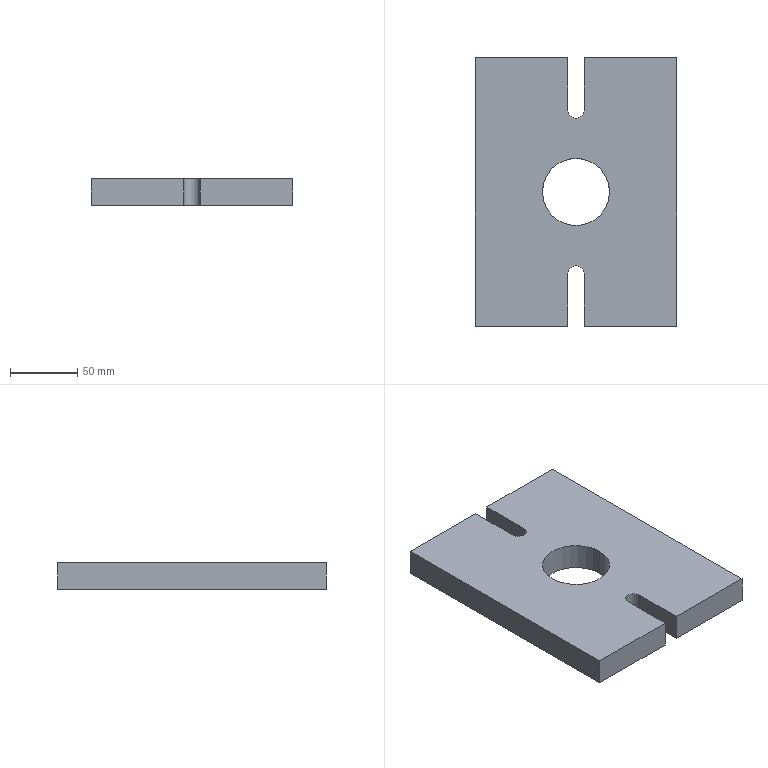Part | SolidWorks | features Extrusion 1 | 1 solid | 16 faces | box 150 x 200 x 20 mm | volume 539748 mm3 | plane 12 | cylinder 4 | commonest cylinder face diameters 12 x2 50 x2
STEP:
#1=CARTESIAN_POINT('',(50.,100.,20.));
#2=VERTEX_POINT('',#1);
#3=CARTESIAN_POINT('',(100.,100.,20.));
#4=VERTEX_POINT('',#3);
#5=CARTESIAN_POINT('',(75.,100.,20.));
#6=DIRECTION('',(0.,0.,1.));
#7=DIRECTION('',(1.,0.,0.));
#8=AXIS2_PLACEMENT_3D('',#5,#6,#7);
#9=CIRCLE('',#8,25.);
#10=EDGE_CURVE('',#2,#4,#9,.T.);
#11=ORIENTED_EDGE('',*,*,#10,.T.);
#12=CARTESIAN_POINT('',(100.,100.,0.));
#13=VERTEX_POINT('',#12);
#14=CARTESIAN_POINT('',(100.,100.,20.));
#15=DIRECTION('',(0.,0.,-1.));
#16=VECTOR('',#15,1000.);
#17=LINE('',#14,#16);
#18=EDGE_CURVE('',#4,#13,#17,.T.);
#19=ORIENTED_EDGE('',*,*,#18,.T.);
#20=CARTESIAN_POINT('',(50.,100.,0.));
#21=VERTEX_POINT('',#20);
#22=CARTESIAN_POINT('',(75.,100.,0.));
#23=DIRECTION('',(0.,0.,1.));
#24=DIRECTION('',(1.,0.,0.));
#25=AXIS2_PLACEMENT_3D('',#22,#23,#24);
#26=CIRCLE('',#25,25.);
#27=EDGE_CURVE('',#21,#13,#26,.T.);
#28=ORIENTED_EDGE('',*,*,#27,.F.);
#29=CARTESIAN_POINT('',(50.,100.,20.));
#30=DIRECTION('',(0.,0.,-1.));
#31=VECTOR('',#30,1000.);
#32=LINE('',#29,#31);
#33=EDGE_CURVE('',#2,#21,#32,.T.);
#34=ORIENTED_EDGE('',*,*,#33,.F.);
#35=EDGE_LOOP('',(#11,#19,#28,#34));
#36=FACE_OUTER_BOUND('',#35,.T.);
#37=CARTESIAN_POINT('',(75.,100.,20.));
#38=DIRECTION('',(0.,0.,-1.));
#39=DIRECTION('',(-1.,0.,0.));
#40=AXIS2_PLACEMENT_3D('',#37,#38,#39);
#41=CYLINDRICAL_SURFACE('',#40,25.);
#42=ADVANCED_FACE('',(#36),#41,.F.);
#43=CARTESIAN_POINT('',(0.,200.,20.));
#44=VERTEX_POINT('',#43);
#45=CARTESIAN_POINT('',(0.,0.,20.));
#46=VERTEX_POINT('',#45);
#47=CARTESIAN_POINT('',(0.,0.,20.));
#48=DIRECTION('',(0.,-1.,0.));
#49=VECTOR('',#48,1000.);
#50=LINE('',#47,#49);
#51=EDGE_CURVE('',#44,#46,#50,.T.);
#52=ORIENTED_EDGE('',*,*,#51,.T.);
#53=CARTESIAN_POINT('',(69.,0.,20.));
#54=VERTEX_POINT('',#53);
#55=CARTESIAN_POINT('',(0.,0.,20.));
#56=DIRECTION('',(1.,0.,0.));
#57=VECTOR('',#56,1000.);
#58=LINE('',#55,#57);
#59=EDGE_CURVE('',#46,#54,#58,.T.);
#60=ORIENTED_EDGE('',*,*,#59,.T.);
#61=CARTESIAN_POINT('',(69.,39.,20.));
#62=VERTEX_POINT('',#61);
#63=CARTESIAN_POINT('',(69.,0.,20.));
#64=DIRECTION('',(0.,1.,0.));
#65=VECTOR('',#64,1000.);
#66=LINE('',#63,#65);
#67=EDGE_CURVE('',#54,#62,#66,.T.);
#68=ORIENTED_EDGE('',*,*,#67,.T.);
#69=CARTESIAN_POINT('',(81.,39.,20.));
#70=VERTEX_POINT('',#69);
#71=CARTESIAN_POINT('',(75.,39.,20.));
#72=DIRECTION('',(0.,0.,-1.));
#73=DIRECTION('',(-1.,0.,0.));
#74=AXIS2_PLACEMENT_3D('',#71,#72,#73);
#75=CIRCLE('',#74,6.);
#76=EDGE_CURVE('',#62,#70,#75,.T.);
#77=ORIENTED_EDGE('',*,*,#76,.T.);
#78=CARTESIAN_POINT('',(81.,0.,20.));
#79=VERTEX_POINT('',#78);
#80=CARTESIAN_POINT('',(81.,39.,20.));
#81=DIRECTION('',(0.,-1.,0.));
#82=VECTOR('',#81,1000.);
#83=LINE('',#80,#82);
#84=EDGE_CURVE('',#70,#79,#83,.T.);
#85=ORIENTED_EDGE('',*,*,#84,.T.);
#86=CARTESIAN_POINT('',(150.,0.,20.));
#87=VERTEX_POINT('',#86);
#88=CARTESIAN_POINT('',(81.,0.,20.));
#89=DIRECTION('',(1.,0.,0.));
#90=VECTOR('',#89,1000.);
#91=LINE('',#88,#90);
#92=EDGE_CURVE('',#79,#87,#91,.T.);
#93=ORIENTED_EDGE('',*,*,#92,.T.);
#94=CARTESIAN_POINT('',(150.,200.,20.));
#95=VERTEX_POINT('',#94);
#96=CARTESIAN_POINT('',(150.,0.,20.));
#97=DIRECTION('',(0.,1.,0.));
#98=VECTOR('',#97,1000.);
#99=LINE('',#96,#98);
#100=EDGE_CURVE('',#87,#95,#99,.T.);
#101=ORIENTED_EDGE('',*,*,#100,.T.);
#102=CARTESIAN_POINT('',(81.,200.,20.));
#103=VERTEX_POINT('',#102);
#104=CARTESIAN_POINT('',(81.,200.,20.));
#105=DIRECTION('',(-1.,0.,0.));
#106=VECTOR('',#105,1000.);
#107=LINE('',#104,#106);
#108=EDGE_CURVE('',#95,#103,#107,.T.);
#109=ORIENTED_EDGE('',*,*,#108,.T.);
#110=CARTESIAN_POINT('',(81.,161.,20.));
#111=VERTEX_POINT('',#110);
#112=CARTESIAN_POINT('',(81.,161.,20.));
#113=DIRECTION('',(0.,-1.,0.));
#114=VECTOR('',#113,1000.);
#115=LINE('',#112,#114);
#116=EDGE_CURVE('',#103,#111,#115,.T.);
#117=ORIENTED_EDGE('',*,*,#116,.T.);
#118=CARTESIAN_POINT('',(69.,161.,20.));
#119=VERTEX_POINT('',#118);
#120=CARTESIAN_POINT('',(75.,161.,20.));
#121=DIRECTION('',(0.,0.,-1.));
#122=DIRECTION('',(1.,0.,0.));
#123=AXIS2_PLACEMENT_3D('',#120,#121,#122);
#124=CIRCLE('',#123,6.);
#125=EDGE_CURVE('',#111,#119,#124,.T.);
#126=ORIENTED_EDGE('',*,*,#125,.T.);
#127=CARTESIAN_POINT('',(69.,200.,20.));
#128=VERTEX_POINT('',#127);
#129=CARTESIAN_POINT('',(69.,200.,20.));
#130=DIRECTION('',(0.,1.,0.));
#131=VECTOR('',#130,1000.);
#132=LINE('',#129,#131);
#133=EDGE_CURVE('',#119,#128,#132,.T.);
#134=ORIENTED_EDGE('',*,*,#133,.T.);
#135=CARTESIAN_POINT('',(0.,200.,20.));
#136=DIRECTION('',(-1.,0.,0.));
#137=VECTOR('',#136,1000.);
#138=LINE('',#135,#137);
#139=EDGE_CURVE('',#128,#44,#138,.T.);
#140=ORIENTED_EDGE('',*,*,#139,.T.);
#141=EDGE_LOOP('',(#52,#60,#68,#77,#85,#93,#101,#109,#117,#126,#134,#140));
#142=FACE_OUTER_BOUND('',#141,.T.);
#143=ORIENTED_EDGE('',*,*,#10,.F.);
#144=CARTESIAN_POINT('',(75.,100.,20.));
#145=DIRECTION('',(0.,0.,1.));
#146=DIRECTION('',(1.,0.,0.));
#147=AXIS2_PLACEMENT_3D('',#144,#145,#146);
#148=CIRCLE('',#147,25.);
#149=EDGE_CURVE('',#4,#2,#148,.T.);
#150=ORIENTED_EDGE('',*,*,#149,.F.);
#151=EDGE_LOOP('',(#143,#150));
#152=FACE_BOUND('',#151,.T.);
#153=CARTESIAN_POINT('',(75.,161.,20.));
#154=DIRECTION('',(0.,0.,1.));
#155=DIRECTION('',(1.,0.,0.));
#156=AXIS2_PLACEMENT_3D('',#153,#154,#155);
#157=PLANE('',#156);
#158=ADVANCED_FACE('',(#142,#152),#157,.T.);
#159=CARTESIAN_POINT('',(0.,200.,0.));
#160=VERTEX_POINT('',#159);
#161=CARTESIAN_POINT('',(0.,0.,0.));
#162=VERTEX_POINT('',#161);
#163=CARTESIAN_POINT('',(0.,0.,0.));
#164=DIRECTION('',(0.,-1.,0.));
#165=VECTOR('',#164,1000.);
#166=LINE('',#163,#165);
#167=EDGE_CURVE('',#160,#162,#166,.T.);
#168=ORIENTED_EDGE('',*,*,#167,.F.);
#169=CARTESIAN_POINT('',(69.,200.,0.));
#170=VERTEX_POINT('',#169);
#171=CARTESIAN_POINT('',(0.,200.,0.));
#172=DIRECTION('',(-1.,0.,0.));
#173=VECTOR('',#172,1000.);
#174=LINE('',#171,#173);
#175=EDGE_CURVE('',#170,#160,#174,.T.);
#176=ORIENTED_EDGE('',*,*,#175,.F.);
#177=CARTESIAN_POINT('',(69.,161.,0.));
#178=VERTEX_POINT('',#177);
#179=CARTESIAN_POINT('',(69.,200.,0.));
#180=DIRECTION('',(0.,1.,0.));
#181=VECTOR('',#180,1000.);
#182=LINE('',#179,#181);
#183=EDGE_CURVE('',#178,#170,#182,.T.);
#184=ORIENTED_EDGE('',*,*,#183,.F.);
#185=CARTESIAN_POINT('',(81.,161.,0.));
#186=VERTEX_POINT('',#185);
#187=CARTESIAN_POINT('',(75.,161.,0.));
#188=DIRECTION('',(0.,0.,-1.));
#189=DIRECTION('',(1.,0.,0.));
#190=AXIS2_PLACEMENT_3D('',#187,#188,#189);
#191=CIRCLE('',#190,6.);
#192=EDGE_CURVE('',#186,#178,#191,.T.);
#193=ORIENTED_EDGE('',*,*,#192,.F.);
#194=CARTESIAN_POINT('',(81.,200.,0.));
#195=VERTEX_POINT('',#194);
#196=CARTESIAN_POINT('',(81.,161.,0.));
#197=DIRECTION('',(0.,-1.,0.));
#198=VECTOR('',#197,1000.);
#199=LINE('',#196,#198);
#200=EDGE_CURVE('',#195,#186,#199,.T.);
#201=ORIENTED_EDGE('',*,*,#200,.F.);
#202=CARTESIAN_POINT('',(150.,200.,0.));
#203=VERTEX_POINT('',#202);
#204=CARTESIAN_POINT('',(81.,200.,0.));
#205=DIRECTION('',(-1.,0.,0.));
#206=VECTOR('',#205,1000.);
#207=LINE('',#204,#206);
#208=EDGE_CURVE('',#203,#195,#207,.T.);
#209=ORIENTED_EDGE('',*,*,#208,.F.);
#210=CARTESIAN_POINT('',(150.,0.,0.));
#211=VERTEX_POINT('',#210);
#212=CARTESIAN_POINT('',(150.,0.,0.));
#213=DIRECTION('',(0.,1.,0.));
#214=VECTOR('',#213,1000.);
#215=LINE('',#212,#214);
#216=EDGE_CURVE('',#211,#203,#215,.T.);
#217=ORIENTED_EDGE('',*,*,#216,.F.);
#218=CARTESIAN_POINT('',(81.,0.,0.));
#219=VERTEX_POINT('',#218);
#220=CARTESIAN_POINT('',(81.,0.,0.));
#221=DIRECTION('',(1.,0.,0.));
#222=VECTOR('',#221,1000.);
#223=LINE('',#220,#222);
#224=EDGE_CURVE('',#219,#211,#223,.T.);
#225=ORIENTED_EDGE('',*,*,#224,.F.);
#226=CARTESIAN_POINT('',(81.,39.,0.));
#227=VERTEX_POINT('',#226);
#228=CARTESIAN_POINT('',(81.,39.,0.));
#229=DIRECTION('',(0.,-1.,0.));
#230=VECTOR('',#229,1000.);
#231=LINE('',#228,#230);
#232=EDGE_CURVE('',#227,#219,#231,.T.);
#233=ORIENTED_EDGE('',*,*,#232,.F.);
#234=CARTESIAN_POINT('',(69.,39.,0.));
#235=VERTEX_POINT('',#234);
#236=CARTESIAN_POINT('',(75.,39.,0.));
#237=DIRECTION('',(0.,0.,-1.));
#238=DIRECTION('',(-1.,0.,0.));
#239=AXIS2_PLACEMENT_3D('',#236,#237,#238);
#240=CIRCLE('',#239,6.);
#241=EDGE_CURVE('',#235,#227,#240,.T.);
#242=ORIENTED_EDGE('',*,*,#241,.F.);
#243=CARTESIAN_POINT('',(69.,0.,0.));
#244=VERTEX_POINT('',#243);
#245=CARTESIAN_POINT('',(69.,0.,0.));
#246=DIRECTION('',(0.,1.,0.));
#247=VECTOR('',#246,1000.);
#248=LINE('',#245,#247);
#249=EDGE_CURVE('',#244,#235,#248,.T.);
#250=ORIENTED_EDGE('',*,*,#249,.F.);
#251=CARTESIAN_POINT('',(0.,0.,0.));
#252=DIRECTION('',(1.,0.,0.));
#253=VECTOR('',#252,1000.);
#254=LINE('',#251,#253);
#255=EDGE_CURVE('',#162,#244,#254,.T.);
#256=ORIENTED_EDGE('',*,*,#255,.F.);
#257=EDGE_LOOP('',(#168,#176,#184,#193,#201,#209,#217,#225,#233,#242,#250,#256));
#258=FACE_OUTER_BOUND('',#257,.T.);
#259=ORIENTED_EDGE('',*,*,#27,.T.);
#260=CARTESIAN_POINT('',(75.,100.,0.));
#261=DIRECTION('',(0.,0.,1.));
#262=DIRECTION('',(1.,0.,0.));
#263=AXIS2_PLACEMENT_3D('',#260,#261,#262);
#264=CIRCLE('',#263,25.);
#265=EDGE_CURVE('',#13,#21,#264,.T.);
#266=ORIENTED_EDGE('',*,*,#265,.T.);
#267=EDGE_LOOP('',(#259,#266));
#268=FACE_BOUND('',#267,.T.);
#269=CARTESIAN_POINT('',(75.,161.,0.));
#270=DIRECTION('',(0.,0.,1.));
#271=DIRECTION('',(1.,0.,0.));
#272=AXIS2_PLACEMENT_3D('',#269,#270,#271);
#273=PLANE('',#272);
#274=ADVANCED_FACE('',(#258,#268),#273,.F.);
#275=ORIENTED_EDGE('',*,*,#167,.T.);
#276=CARTESIAN_POINT('',(0.,0.,20.));
#277=DIRECTION('',(0.,0.,-1.));
#278=VECTOR('',#277,1000.);
#279=LINE('',#276,#278);
#280=EDGE_CURVE('',#46,#162,#279,.T.);
#281=ORIENTED_EDGE('',*,*,#280,.F.);
#282=ORIENTED_EDGE('',*,*,#51,.F.);
#283=CARTESIAN_POINT('',(0.,200.,20.));
#284=DIRECTION('',(0.,0.,-1.));
#285=VECTOR('',#284,1000.);
#286=LINE('',#283,#285);
#287=EDGE_CURVE('',#44,#160,#286,.T.);
#288=ORIENTED_EDGE('',*,*,#287,.T.);
#289=EDGE_LOOP('',(#275,#281,#282,#288));
#290=FACE_OUTER_BOUND('',#289,.T.);
#291=CARTESIAN_POINT('',(0.,0.,20.));
#292=DIRECTION('',(1.,0.,0.));
#293=DIRECTION('',(0.,0.,-1.));
#294=AXIS2_PLACEMENT_3D('',#291,#292,#293);
#295=PLANE('',#294);
#296=ADVANCED_FACE('',(#290),#295,.F.);
#297=ORIENTED_EDGE('',*,*,#255,.T.);
#298=CARTESIAN_POINT('',(69.,0.,20.));
#299=DIRECTION('',(0.,0.,-1.));
#300=VECTOR('',#299,1000.);
#301=LINE('',#298,#300);
#302=EDGE_CURVE('',#54,#244,#301,.T.);
#303=ORIENTED_EDGE('',*,*,#302,.F.);
#304=ORIENTED_EDGE('',*,*,#59,.F.);
#305=ORIENTED_EDGE('',*,*,#280,.T.);
#306=EDGE_LOOP('',(#297,#303,#304,#305));
#307=FACE_OUTER_BOUND('',#306,.T.);
#308=CARTESIAN_POINT('',(0.,0.,20.));
#309=DIRECTION('',(0.,1.,0.));
#310=DIRECTION('',(0.,0.,1.));
#311=AXIS2_PLACEMENT_3D('',#308,#309,#310);
#312=PLANE('',#311);
#313=ADVANCED_FACE('',(#307),#312,.F.);
#314=ORIENTED_EDGE('',*,*,#249,.T.);
#315=CARTESIAN_POINT('',(69.,39.,20.));
#316=DIRECTION('',(0.,0.,-1.));
#317=VECTOR('',#316,1000.);
#318=LINE('',#315,#317);
#319=EDGE_CURVE('',#62,#235,#318,.T.);
#320=ORIENTED_EDGE('',*,*,#319,.F.);
#321=ORIENTED_EDGE('',*,*,#67,.F.);
#322=ORIENTED_EDGE('',*,*,#302,.T.);
#323=EDGE_LOOP('',(#314,#320,#321,#322));
#324=FACE_OUTER_BOUND('',#323,.T.);
#325=CARTESIAN_POINT('',(69.,0.,20.));
#326=DIRECTION('',(-1.,0.,0.));
#327=DIRECTION('',(0.,-1.,0.));
#328=AXIS2_PLACEMENT_3D('',#325,#326,#327);
#329=PLANE('',#328);
#330=ADVANCED_FACE('',(#324),#329,.F.);
#331=ORIENTED_EDGE('',*,*,#241,.T.);
#332=CARTESIAN_POINT('',(81.,39.,20.));
#333=DIRECTION('',(0.,0.,-1.));
#334=VECTOR('',#333,1000.);
#335=LINE('',#332,#334);
#336=EDGE_CURVE('',#70,#227,#335,.T.);
#337=ORIENTED_EDGE('',*,*,#336,.F.);
#338=ORIENTED_EDGE('',*,*,#76,.F.);
#339=ORIENTED_EDGE('',*,*,#319,.T.);
#340=EDGE_LOOP('',(#331,#337,#338,#339));
#341=FACE_OUTER_BOUND('',#340,.T.);
#342=CARTESIAN_POINT('',(75.,39.,20.));
#343=DIRECTION('',(0.,0.,-1.));
#344=DIRECTION('',(-1.,0.,0.));
#345=AXIS2_PLACEMENT_3D('',#342,#343,#344);
#346=CYLINDRICAL_SURFACE('',#345,6.);
#347=ADVANCED_FACE('',(#341),#346,.F.);
#348=ORIENTED_EDGE('',*,*,#232,.T.);
#349=CARTESIAN_POINT('',(81.,0.,20.));
#350=DIRECTION('',(0.,0.,-1.));
#351=VECTOR('',#350,1000.);
#352=LINE('',#349,#351);
#353=EDGE_CURVE('',#79,#219,#352,.T.);
#354=ORIENTED_EDGE('',*,*,#353,.F.);
#355=ORIENTED_EDGE('',*,*,#84,.F.);
#356=ORIENTED_EDGE('',*,*,#336,.T.);
#357=EDGE_LOOP('',(#348,#354,#355,#356));
#358=FACE_OUTER_BOUND('',#357,.T.);
#359=CARTESIAN_POINT('',(81.,39.,20.));
#360=DIRECTION('',(1.,0.,0.));
#361=DIRECTION('',(0.,0.,-1.));
#362=AXIS2_PLACEMENT_3D('',#359,#360,#361);
#363=PLANE('',#362);
#364=ADVANCED_FACE('',(#358),#363,.F.);
#365=ORIENTED_EDGE('',*,*,#224,.T.);
#366=CARTESIAN_POINT('',(150.,0.,20.));
#367=DIRECTION('',(0.,0.,-1.));
#368=VECTOR('',#367,1000.);
#369=LINE('',#366,#368);
#370=EDGE_CURVE('',#87,#211,#369,.T.);
#371=ORIENTED_EDGE('',*,*,#370,.F.);
#372=ORIENTED_EDGE('',*,*,#92,.F.);
#373=ORIENTED_EDGE('',*,*,#353,.T.);
#374=EDGE_LOOP('',(#365,#371,#372,#373));
#375=FACE_OUTER_BOUND('',#374,.T.);
#376=CARTESIAN_POINT('',(81.,0.,20.));
#377=DIRECTION('',(0.,1.,0.));
#378=DIRECTION('',(-1.,0.,0.));
#379=AXIS2_PLACEMENT_3D('',#376,#377,#378);
#380=PLANE('',#379);
#381=ADVANCED_FACE('',(#375),#380,.F.);
#382=ORIENTED_EDGE('',*,*,#216,.T.);
#383=CARTESIAN_POINT('',(150.,200.,20.));
#384=DIRECTION('',(0.,0.,-1.));
#385=VECTOR('',#384,1000.);
#386=LINE('',#383,#385);
#387=EDGE_CURVE('',#95,#203,#386,.T.);
#388=ORIENTED_EDGE('',*,*,#387,.F.);
#389=ORIENTED_EDGE('',*,*,#100,.F.);
#390=ORIENTED_EDGE('',*,*,#370,.T.);
#391=EDGE_LOOP('',(#382,#388,#389,#390));
#392=FACE_OUTER_BOUND('',#391,.T.);
#393=CARTESIAN_POINT('',(150.,0.,20.));
#394=DIRECTION('',(-1.,0.,0.));
#395=DIRECTION('',(0.,0.,1.));
#396=AXIS2_PLACEMENT_3D('',#393,#394,#395);
#397=PLANE('',#396);
#398=ADVANCED_FACE('',(#392),#397,.F.);
#399=ORIENTED_EDGE('',*,*,#208,.T.);
#400=CARTESIAN_POINT('',(81.,200.,20.));
#401=DIRECTION('',(0.,0.,-1.));
#402=VECTOR('',#401,1000.);
#403=LINE('',#400,#402);
#404=EDGE_CURVE('',#103,#195,#403,.T.);
#405=ORIENTED_EDGE('',*,*,#404,.F.);
#406=ORIENTED_EDGE('',*,*,#108,.F.);
#407=ORIENTED_EDGE('',*,*,#387,.T.);
#408=EDGE_LOOP('',(#399,#405,#406,#407));
#409=FACE_OUTER_BOUND('',#408,.T.);
#410=CARTESIAN_POINT('',(81.,200.,20.));
#411=DIRECTION('',(0.,-1.,0.));
#412=DIRECTION('',(0.,0.,-1.));
#413=AXIS2_PLACEMENT_3D('',#410,#411,#412);
#414=PLANE('',#413);
#415=ADVANCED_FACE('',(#409),#414,.F.);
#416=ORIENTED_EDGE('',*,*,#200,.T.);
#417=CARTESIAN_POINT('',(81.,161.,20.));
#418=DIRECTION('',(0.,0.,-1.));
#419=VECTOR('',#418,1000.);
#420=LINE('',#417,#419);
#421=EDGE_CURVE('',#111,#186,#420,.T.);
#422=ORIENTED_EDGE('',*,*,#421,.F.);
#423=ORIENTED_EDGE('',*,*,#116,.F.);
#424=ORIENTED_EDGE('',*,*,#404,.T.);
#425=EDGE_LOOP('',(#416,#422,#423,#424));
#426=FACE_OUTER_BOUND('',#425,.T.);
#427=CARTESIAN_POINT('',(81.,161.,20.));
#428=DIRECTION('',(1.,0.,0.));
#429=DIRECTION('',(0.,0.,-1.));
#430=AXIS2_PLACEMENT_3D('',#427,#428,#429);
#431=PLANE('',#430);
#432=ADVANCED_FACE('',(#426),#431,.F.);
#433=ORIENTED_EDGE('',*,*,#192,.T.);
#434=CARTESIAN_POINT('',(69.,161.,20.));
#435=DIRECTION('',(0.,0.,-1.));
#436=VECTOR('',#435,1000.);
#437=LINE('',#434,#436);
#438=EDGE_CURVE('',#119,#178,#437,.T.);
#439=ORIENTED_EDGE('',*,*,#438,.F.);
#440=ORIENTED_EDGE('',*,*,#125,.F.);
#441=ORIENTED_EDGE('',*,*,#421,.T.);
#442=EDGE_LOOP('',(#433,#439,#440,#441));
#443=FACE_OUTER_BOUND('',#442,.T.);
#444=CARTESIAN_POINT('',(75.,161.,20.));
#445=DIRECTION('',(0.,0.,-1.));
#446=DIRECTION('',(-1.,0.,0.));
#447=AXIS2_PLACEMENT_3D('',#444,#445,#446);
#448=CYLINDRICAL_SURFACE('',#447,6.);
#449=ADVANCED_FACE('',(#443),#448,.F.);
#450=ORIENTED_EDGE('',*,*,#183,.T.);
#451=CARTESIAN_POINT('',(69.,200.,20.));
#452=DIRECTION('',(0.,0.,-1.));
#453=VECTOR('',#452,1000.);
#454=LINE('',#451,#453);
#455=EDGE_CURVE('',#128,#170,#454,.T.);
#456=ORIENTED_EDGE('',*,*,#455,.F.);
#457=ORIENTED_EDGE('',*,*,#133,.F.);
#458=ORIENTED_EDGE('',*,*,#438,.T.);
#459=EDGE_LOOP('',(#450,#456,#457,#458));
#460=FACE_OUTER_BOUND('',#459,.T.);
#461=CARTESIAN_POINT('',(69.,200.,20.));
#462=DIRECTION('',(-1.,0.,0.));
#463=DIRECTION('',(0.,-1.,0.));
#464=AXIS2_PLACEMENT_3D('',#461,#462,#463);
#465=PLANE('',#464);
#466=ADVANCED_FACE('',(#460),#465,.F.);
#467=ORIENTED_EDGE('',*,*,#175,.T.);
#468=ORIENTED_EDGE('',*,*,#287,.F.);
#469=ORIENTED_EDGE('',*,*,#139,.F.);
#470=ORIENTED_EDGE('',*,*,#455,.T.);
#471=EDGE_LOOP('',(#467,#468,#469,#470));
#472=FACE_OUTER_BOUND('',#471,.T.);
#473=CARTESIAN_POINT('',(0.,200.,20.));
#474=DIRECTION('',(0.,-1.,0.));
#475=DIRECTION('',(0.,0.,-1.));
#476=AXIS2_PLACEMENT_3D('',#473,#474,#475);
#477=PLANE('',#476);
#478=ADVANCED_FACE('',(#472),#477,.F.);
#479=ORIENTED_EDGE('',*,*,#18,.F.);
#480=ORIENTED_EDGE('',*,*,#149,.T.);
#481=ORIENTED_EDGE('',*,*,#33,.T.);
#482=ORIENTED_EDGE('',*,*,#265,.F.);
#483=EDGE_LOOP('',(#479,#480,#481,#482));
#484=FACE_OUTER_BOUND('',#483,.T.);
#485=CARTESIAN_POINT('',(75.,100.,20.));
#486=DIRECTION('',(0.,0.,-1.));
#487=DIRECTION('',(-1.,0.,0.));
#488=AXIS2_PLACEMENT_3D('',#485,#486,#487);
#489=CYLINDRICAL_SURFACE('',#488,25.);
#490=ADVANCED_FACE('',(#484),#489,.F.);
#491=CLOSED_SHELL('',(#42,#158,#274,#296,#313,#330,#347,#364,#381,#398,#415,#432,#449,#466,#478,#490));
#492=MANIFOLD_SOLID_BREP('',#491);
#493=CARTESIAN_POINT('',(0.,0.,0.));
#494=DIRECTION('',(0.,0.,1.));
#495=DIRECTION('',(1.,0.,0.));
#496=AXIS2_PLACEMENT_3D('',#493,#494,#495);
#497=(LENGTH_UNIT()NAMED_UNIT(*)SI_UNIT(.MILLI.,.METRE.));
#498=UNCERTAINTY_MEASURE_WITH_UNIT(LENGTH_MEASURE(0.00001),#497,'','');
#499=(NAMED_UNIT(*)PLANE_ANGLE_UNIT()SI_UNIT($,.RADIAN.));
#500=(NAMED_UNIT(*)SI_UNIT($,.STERADIAN.)SOLID_ANGLE_UNIT());
#501=(GEOMETRIC_REPRESENTATION_CONTEXT(3)GLOBAL_UNCERTAINTY_ASSIGNED_CONTEXT((#498))GLOBAL_UNIT_ASSIGNED_CONTEXT((#497,#499,#500))REPRESENTATION_CONTEXT('',''));
#502=ADVANCED_BREP_SHAPE_REPRESENTATION('',(#492,#496),#501);